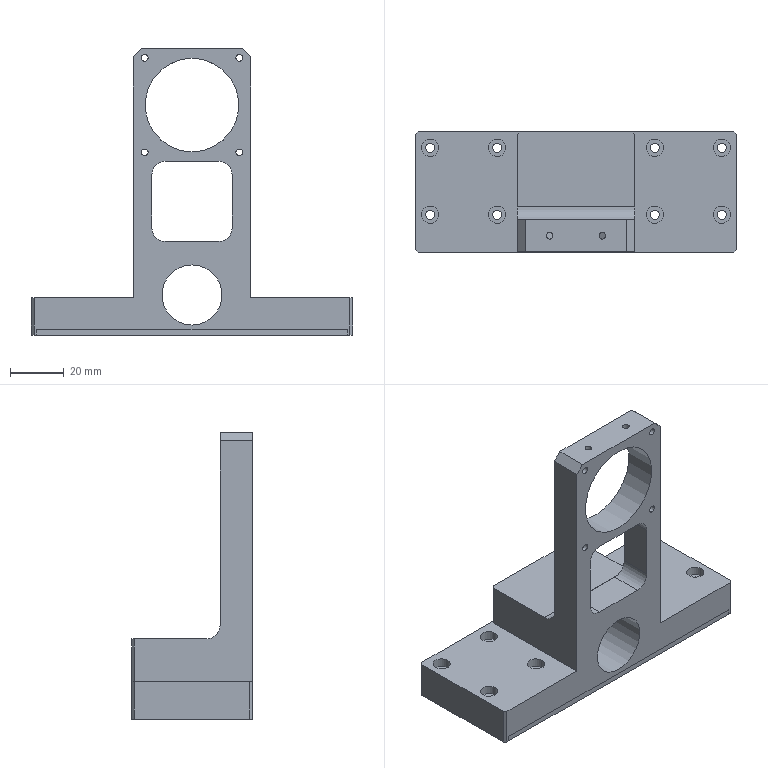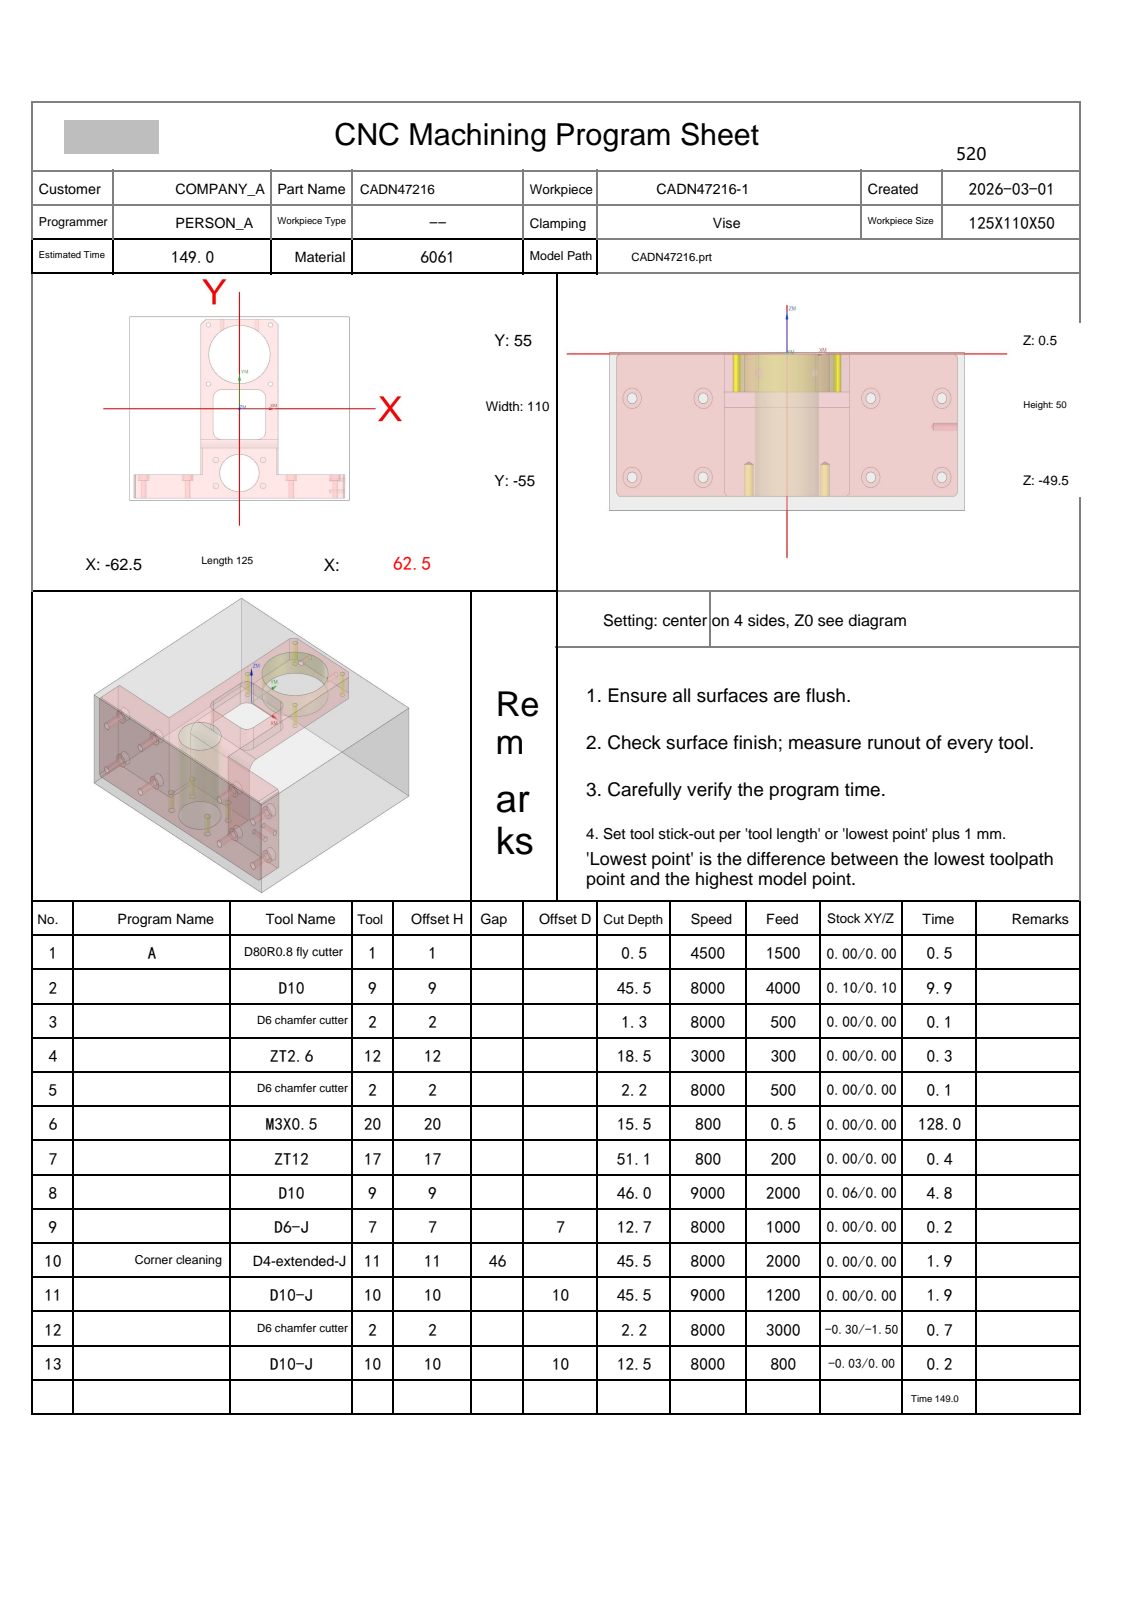NC program | NX | posted by the shop | part box 120 x 45 x 107 mm
Lines 6509 to 7503 of 16292:
N10 T11 M06
(D4-extended-J  D=4. R=0. H=11 ce=0.00 di=0.00)
G00 G90 G54 X-27.403 Y-37.1 M03 S8000
G43 H11 Z50.
M08
Z.15
G01 X-27.402 Y-37.105 Z.089 F2000.
X-27.398 Y-37.119 Z.034
X-27.392 Y-37.142 Z-.014
X-27.383 Y-37.17 Z-.058
X-27.37 Y-37.204 Z-.096
X-27.354 Y-37.241 Z-.129
X-27.334 Y-37.28 Z-.157
X-27.31 Y-37.32 Z-.181
X-27.282 Y-37.359 Z-.201
X-27.249 Y-37.396 Z-.217
X-27.211 Y-37.43 Z-.23
X-27.167 Y-37.458 Z-.239
X-27.119 Y-37.481 Z-.245
X-27.064 Y-37.495 Z-.249
X-27.003 Y-37.5 Z-.25
X-24.
Y-34.497
X-24.014 Y-34.454 Z-.251
X-24.053 Y-34.433 Z-.253
X-24.116 Y-34.432 Z-.256
X-24.199 Y-34.45 Z-.261
X-24.299 Y-34.485 Z-.267
X-24.414 Y-34.535 Z-.274
X-24.541 Y-34.599 Z-.281
X-24.677 Y-34.675 Z-.29
X-24.896 Y-34.812 Z-.303
X-25.113 Y-34.96 Z-.318
X-25.509 Y-35.271 Z-.346
X-25.883 Y-35.617 Z-.375
X-26.229 Y-35.991 Z-.404
X-26.54 Y-36.387 Z-.432
X-26.688 Y-36.604 Z-.447
X-26.825 Y-36.823 Z-.46
X-26.901 Y-36.959 Z-.469
X-26.965 Y-37.086 Z-.476
X-27.015 Y-37.201 Z-.483
X-27.05 Y-37.301 Z-.489
X-27.068 Y-37.384 Z-.494
X-27.067 Y-37.447 Z-.497
X-27.046 Y-37.486 Z-.499
X-27.003 Y-37.5 Z-.5
X-24.
Y-34.497
X-24.014 Y-34.454 Z-.501
X-24.053 Y-34.433 Z-.503
X-24.116 Y-34.432 Z-.506
X-24.199 Y-34.45 Z-.511
X-24.299 Y-34.485 Z-.517
X-24.414 Y-34.535 Z-.524
X-24.541 Y-34.599 Z-.531
X-24.677 Y-34.675 Z-.54
X-24.896 Y-34.812 Z-.553
X-25.113 Y-34.96 Z-.568
X-25.509 Y-35.271 Z-.596
X-25.883 Y-35.617 Z-.625
X-26.229 Y-35.991 Z-.654
X-26.54 Y-36.387 Z-.682
X-26.688 Y-36.604 Z-.697
X-26.825 Y-36.823 Z-.71
X-26.901 Y-36.959 Z-.719
X-26.965 Y-37.086 Z-.726
X-27.015 Y-37.201 Z-.733
X-27.05 Y-37.301 Z-.739
X-27.068 Y-37.384 Z-.744
X-27.067 Y-37.447 Z-.747
X-27.046 Y-37.486 Z-.749
X-27.003 Y-37.5 Z-.75
X-24.
Y-34.497
X-24.014 Y-34.454 Z-.751
X-24.053 Y-34.433 Z-.753
X-24.116 Y-34.432 Z-.756
X-24.199 Y-34.45 Z-.761
X-24.299 Y-34.485 Z-.767
X-24.414 Y-34.535 Z-.774
X-24.541 Y-34.599 Z-.781
X-24.677 Y-34.675 Z-.79
X-24.896 Y-34.812 Z-.803
X-25.113 Y-34.96 Z-.818
X-25.509 Y-35.271 Z-.846
X-25.883 Y-35.617 Z-.875
X-26.229 Y-35.991 Z-.904
X-26.54 Y-36.387 Z-.932
X-26.688 Y-36.604 Z-.947
X-26.825 Y-36.823 Z-.96
X-26.901 Y-36.959 Z-.969
X-26.965 Y-37.086 Z-.976
X-27.015 Y-37.201 Z-.983
X-27.05 Y-37.301 Z-.989
X-27.068 Y-37.384 Z-.994
X-27.067 Y-37.447 Z-.997
X-27.046 Y-37.486 Z-.999
X-27.003 Y-37.5 Z-1.
X-24.
Y-34.497
X-24.014 Y-34.454 Z-1.001
X-24.053 Y-34.433 Z-1.003
X-24.116 Y-34.432 Z-1.006
X-24.199 Y-34.45 Z-1.011
X-24.299 Y-34.485 Z-1.017
X-24.414 Y-34.535 Z-1.024
X-24.541 Y-34.599 Z-1.031
X-24.677 Y-34.675 Z-1.04
X-24.896 Y-34.811 Z-1.053
X-25.113 Y-34.96 Z-1.068
X-25.509 Y-35.271 Z-1.096
X-25.883 Y-35.617 Z-1.125
X-26.229 Y-35.991 Z-1.154
X-26.54 Y-36.386 Z-1.182
X-26.688 Y-36.604 Z-1.197
X-26.825 Y-36.823 Z-1.21
X-26.901 Y-36.959 Z-1.219
X-26.965 Y-37.086 Z-1.226
X-27.015 Y-37.201 Z-1.233
X-27.05 Y-37.301 Z-1.239
X-27.068 Y-37.384 Z-1.244
X-27.067 Y-37.447 Z-1.247
X-27.046 Y-37.486 Z-1.249
X-27.003 Y-37.5 Z-1.25
X-24.
Y-34.497
X-24.014 Y-34.454 Z-1.251
X-24.053 Y-34.433 Z-1.253
X-24.116 Y-34.432 Z-1.256
X-24.199 Y-34.45 Z-1.261
X-24.299 Y-34.485 Z-1.267
X-24.414 Y-34.535 Z-1.274
X-24.541 Y-34.599 Z-1.281
X-24.677 Y-34.675 Z-1.29
X-24.896 Y-34.811 Z-1.303
X-25.113 Y-34.96 Z-1.318
X-25.509 Y-35.271 Z-1.346
X-25.883 Y-35.617 Z-1.375
X-26.229 Y-35.991 Z-1.404
X-26.54 Y-36.386 Z-1.432
X-26.688 Y-36.604 Z-1.447
X-26.825 Y-36.823 Z-1.46
X-26.901 Y-36.959 Z-1.469
X-26.965 Y-37.086 Z-1.476
X-27.015 Y-37.201 Z-1.483
X-27.05 Y-37.301 Z-1.489
X-27.068 Y-37.384 Z-1.494
X-27.067 Y-37.447 Z-1.497
X-27.046 Y-37.486 Z-1.499
X-27.003 Y-37.5 Z-1.5
X-24.
Y-34.497
X-24.014 Y-34.454 Z-1.501
X-24.053 Y-34.433 Z-1.503
X-24.116 Y-34.432 Z-1.506
X-24.199 Y-34.45 Z-1.511
X-24.299 Y-34.485 Z-1.517
X-24.414 Y-34.535 Z-1.524
X-24.541 Y-34.599 Z-1.531
X-24.677 Y-34.675 Z-1.54
X-24.896 Y-34.811 Z-1.553
X-25.113 Y-34.96 Z-1.568
X-25.509 Y-35.271 Z-1.596
X-25.883 Y-35.617 Z-1.625
X-26.229 Y-35.991 Z-1.654
X-26.54 Y-36.386 Z-1.682
X-26.688 Y-36.604 Z-1.697
X-26.825 Y-36.823 Z-1.71
X-26.901 Y-36.959 Z-1.719
X-26.965 Y-37.086 Z-1.726
X-27.015 Y-37.201 Z-1.733
X-27.05 Y-37.301 Z-1.739
X-27.068 Y-37.384 Z-1.744
X-27.067 Y-37.447 Z-1.747
X-27.046 Y-37.486 Z-1.749
X-27.003 Y-37.5 Z-1.75
X-24.
Y-34.497
X-24.014 Y-34.454 Z-1.751
X-24.053 Y-34.433 Z-1.753
X-24.116 Y-34.432 Z-1.756
X-24.199 Y-34.45 Z-1.761
X-24.299 Y-34.485 Z-1.767
X-24.414 Y-34.535 Z-1.774
X-24.541 Y-34.599 Z-1.781
X-24.677 Y-34.675 Z-1.79
X-24.896 Y-34.811 Z-1.803
X-25.113 Y-34.96 Z-1.818
X-25.509 Y-35.271 Z-1.846
X-25.883 Y-35.617 Z-1.875
X-26.229 Y-35.991 Z-1.904
X-26.54 Y-36.386 Z-1.932
X-26.688 Y-36.604 Z-1.947
X-26.825 Y-36.823 Z-1.96
X-26.901 Y-36.959 Z-1.969
X-26.965 Y-37.086 Z-1.976
X-27.015 Y-37.201 Z-1.983
X-27.05 Y-37.301 Z-1.989
X-27.068 Y-37.384 Z-1.994
X-27.067 Y-37.447 Z-1.997
X-27.046 Y-37.486 Z-1.999
X-27.003 Y-37.5 Z-2.
X-24.
Y-34.497
X-24.014 Y-34.454 Z-2.001
X-24.053 Y-34.433 Z-2.003
X-24.116 Y-34.432 Z-2.006
X-24.199 Y-34.45 Z-2.011
X-24.299 Y-34.485 Z-2.017
X-24.414 Y-34.535 Z-2.024
X-24.541 Y-34.599 Z-2.031
X-24.677 Y-34.675 Z-2.04
X-24.896 Y-34.811 Z-2.053
X-25.113 Y-34.96 Z-2.068
X-25.509 Y-35.271 Z-2.096
X-25.883 Y-35.617 Z-2.125
X-26.229 Y-35.991 Z-2.154
X-26.54 Y-36.386 Z-2.182
X-26.688 Y-36.604 Z-2.197
X-26.825 Y-36.823 Z-2.21
X-26.901 Y-36.959 Z-2.219
X-26.965 Y-37.086 Z-2.226
X-27.015 Y-37.201 Z-2.233
X-27.05 Y-37.301 Z-2.239
X-27.068 Y-37.384 Z-2.244
X-27.067 Y-37.447 Z-2.247
X-27.046 Y-37.486 Z-2.249
X-27.003 Y-37.5 Z-2.25
X-24.
Y-34.497
X-24.014 Y-34.454 Z-2.251
X-24.053 Y-34.433 Z-2.253
X-24.116 Y-34.432 Z-2.256
X-24.199 Y-34.45 Z-2.261
X-24.299 Y-34.485 Z-2.267
X-24.414 Y-34.535 Z-2.274
X-24.541 Y-34.599 Z-2.281
X-24.677 Y-34.675 Z-2.29
X-24.896 Y-34.811 Z-2.303
X-25.113 Y-34.96 Z-2.318
X-25.509 Y-35.271 Z-2.346
X-25.883 Y-35.617 Z-2.375
X-26.229 Y-35.991 Z-2.404
X-26.54 Y-36.386 Z-2.432
X-26.688 Y-36.604 Z-2.447
X-26.825 Y-36.823 Z-2.46
X-26.901 Y-36.959 Z-2.469
X-26.965 Y-37.086 Z-2.476
X-27.015 Y-37.201 Z-2.483
X-27.05 Y-37.301 Z-2.489
X-27.068 Y-37.384 Z-2.494
X-27.067 Y-37.447 Z-2.497
X-27.046 Y-37.486 Z-2.499
X-27.003 Y-37.5 Z-2.5
X-24.
Y-34.497
X-24.014 Y-34.454 Z-2.501
X-24.053 Y-34.433 Z-2.503
X-24.116 Y-34.432 Z-2.506
X-24.199 Y-34.45 Z-2.511
X-24.299 Y-34.485 Z-2.517
X-24.414 Y-34.535 Z-2.524
X-24.541 Y-34.599 Z-2.531
X-24.677 Y-34.675 Z-2.54
X-24.896 Y-34.811 Z-2.553
X-25.113 Y-34.96 Z-2.568
X-25.509 Y-35.271 Z-2.596
X-25.883 Y-35.617 Z-2.625
X-26.229 Y-35.991 Z-2.654
X-26.54 Y-36.386 Z-2.682
X-26.688 Y-36.604 Z-2.697
X-26.825 Y-36.823 Z-2.71
X-26.901 Y-36.959 Z-2.719
X-26.965 Y-37.086 Z-2.726
X-27.015 Y-37.201 Z-2.733
X-27.05 Y-37.301 Z-2.739
X-27.068 Y-37.384 Z-2.744
X-27.067 Y-37.447 Z-2.747
X-27.046 Y-37.486 Z-2.749
X-27.003 Y-37.5 Z-2.75
X-24.
Y-34.497
X-24.014 Y-34.454 Z-2.751
X-24.053 Y-34.433 Z-2.753
X-24.116 Y-34.432 Z-2.756
X-24.199 Y-34.45 Z-2.761
X-24.299 Y-34.485 Z-2.767
X-24.414 Y-34.535 Z-2.774
X-24.541 Y-34.599 Z-2.781
X-24.677 Y-34.675 Z-2.79
X-24.896 Y-34.811 Z-2.803
X-25.113 Y-34.96 Z-2.818
X-25.509 Y-35.271 Z-2.846
X-25.883 Y-35.617 Z-2.875
X-26.229 Y-35.991 Z-2.904
X-26.54 Y-36.386 Z-2.932
X-26.688 Y-36.604 Z-2.947
X-26.825 Y-36.823 Z-2.96
X-26.901 Y-36.959 Z-2.969
X-26.965 Y-37.086 Z-2.976
X-27.015 Y-37.201 Z-2.983
X-27.05 Y-37.301 Z-2.989
X-27.068 Y-37.384 Z-2.994
X-27.067 Y-37.447 Z-2.997
X-27.046 Y-37.486 Z-2.999
X-27.003 Y-37.5 Z-3.
X-24.
Y-34.497
X-24.014 Y-34.454 Z-3.001
X-24.053 Y-34.433 Z-3.003
X-24.116 Y-34.432 Z-3.006
X-24.199 Y-34.45 Z-3.011
X-24.299 Y-34.485 Z-3.017
X-24.414 Y-34.535 Z-3.024
X-24.541 Y-34.599 Z-3.031
X-24.677 Y-34.675 Z-3.04
X-24.896 Y-34.811 Z-3.053
X-25.113 Y-34.96 Z-3.068
X-25.509 Y-35.271 Z-3.096
X-25.883 Y-35.617 Z-3.125
X-26.229 Y-35.991 Z-3.154
X-26.54 Y-36.386 Z-3.182
X-26.688 Y-36.604 Z-3.197
X-26.825 Y-36.823 Z-3.21
X-26.901 Y-36.959 Z-3.219
X-26.965 Y-37.086 Z-3.226
X-27.015 Y-37.201 Z-3.233
X-27.05 Y-37.301 Z-3.239
X-27.068 Y-37.384 Z-3.244
X-27.067 Y-37.447 Z-3.247
X-27.046 Y-37.486 Z-3.249
X-27.003 Y-37.5 Z-3.25
X-24.
Y-34.497
X-24.014 Y-34.454 Z-3.251
X-24.053 Y-34.433 Z-3.253
X-24.116 Y-34.432 Z-3.256
X-24.199 Y-34.45 Z-3.261
X-24.299 Y-34.485 Z-3.267
X-24.414 Y-34.535 Z-3.274
X-24.541 Y-34.599 Z-3.281
X-24.677 Y-34.675 Z-3.29
X-24.896 Y-34.811 Z-3.303
X-25.113 Y-34.96 Z-3.318
X-25.509 Y-35.271 Z-3.346
X-25.883 Y-35.617 Z-3.375
X-26.229 Y-35.991 Z-3.404
X-26.54 Y-36.386 Z-3.432
X-26.688 Y-36.604 Z-3.447
X-26.825 Y-36.823 Z-3.46
X-26.901 Y-36.959 Z-3.469
X-26.965 Y-37.086 Z-3.476
X-27.015 Y-37.201 Z-3.483
X-27.05 Y-37.301 Z-3.489
X-27.068 Y-37.384 Z-3.494
X-27.067 Y-37.447 Z-3.497
X-27.046 Y-37.486 Z-3.499
X-27.003 Y-37.5 Z-3.5
X-24.
Y-34.497
X-24.014 Y-34.454 Z-3.501
X-24.053 Y-34.433 Z-3.503
X-24.116 Y-34.432 Z-3.506
X-24.199 Y-34.45 Z-3.511
X-24.299 Y-34.485 Z-3.517
X-24.414 Y-34.535 Z-3.524
X-24.541 Y-34.599 Z-3.531
X-24.677 Y-34.675 Z-3.54
X-24.896 Y-34.811 Z-3.553
X-25.113 Y-34.96 Z-3.568
X-25.509 Y-35.271 Z-3.596
X-25.883 Y-35.617 Z-3.625
X-26.229 Y-35.991 Z-3.654
X-26.54 Y-36.386 Z-3.682
X-26.688 Y-36.604 Z-3.697
X-26.825 Y-36.823 Z-3.71
X-26.901 Y-36.959 Z-3.719
X-26.965 Y-37.086 Z-3.726
X-27.015 Y-37.201 Z-3.733
X-27.05 Y-37.301 Z-3.739
X-27.068 Y-37.384 Z-3.744
X-27.067 Y-37.447 Z-3.747
X-27.046 Y-37.486 Z-3.749
X-27.003 Y-37.5 Z-3.75
X-24.
Y-34.497
X-24.014 Y-34.454 Z-3.751
X-24.053 Y-34.433 Z-3.753
X-24.116 Y-34.432 Z-3.756
X-24.199 Y-34.45 Z-3.761
X-24.299 Y-34.485 Z-3.767
X-24.414 Y-34.535 Z-3.774
X-24.541 Y-34.599 Z-3.781
X-24.677 Y-34.675 Z-3.79
X-24.896 Y-34.811 Z-3.803
X-25.113 Y-34.96 Z-3.818
X-25.509 Y-35.271 Z-3.846
X-25.883 Y-35.617 Z-3.875
X-26.229 Y-35.991 Z-3.904
X-26.54 Y-36.386 Z-3.932
X-26.688 Y-36.604 Z-3.947
X-26.825 Y-36.823 Z-3.96
X-26.901 Y-36.959 Z-3.969
X-26.965 Y-37.086 Z-3.976
X-27.015 Y-37.201 Z-3.983
X-27.05 Y-37.301 Z-3.989
X-27.068 Y-37.384 Z-3.994
X-27.067 Y-37.447 Z-3.997
X-27.046 Y-37.486 Z-3.999
X-27.003 Y-37.5 Z-4.
X-24.
Y-34.497
X-24.014 Y-34.454 Z-4.001
X-24.053 Y-34.433 Z-4.003
X-24.116 Y-34.432 Z-4.006
X-24.199 Y-34.45 Z-4.011
X-24.299 Y-34.485 Z-4.017
X-24.414 Y-34.535 Z-4.024
X-24.541 Y-34.599 Z-4.031
X-24.677 Y-34.675 Z-4.04
X-24.896 Y-34.811 Z-4.053
X-25.113 Y-34.96 Z-4.068
X-25.509 Y-35.271 Z-4.096
X-25.883 Y-35.617 Z-4.125
X-26.229 Y-35.991 Z-4.154
X-26.54 Y-36.386 Z-4.182
X-26.688 Y-36.604 Z-4.197
X-26.825 Y-36.823 Z-4.21
X-26.901 Y-36.959 Z-4.219
X-26.965 Y-37.086 Z-4.226
X-27.015 Y-37.201 Z-4.233
X-27.05 Y-37.301 Z-4.239
X-27.068 Y-37.384 Z-4.244
X-27.067 Y-37.447 Z-4.247
X-27.046 Y-37.486 Z-4.249
X-27.003 Y-37.5 Z-4.25
X-24.
Y-34.497
X-24.014 Y-34.454 Z-4.251
X-24.053 Y-34.433 Z-4.253
X-24.116 Y-34.432 Z-4.256
X-24.199 Y-34.45 Z-4.261
X-24.299 Y-34.485 Z-4.267
X-24.414 Y-34.535 Z-4.274
X-24.541 Y-34.599 Z-4.281
X-24.677 Y-34.675 Z-4.29
X-24.896 Y-34.811 Z-4.303
X-25.113 Y-34.96 Z-4.318
X-25.509 Y-35.271 Z-4.346
X-25.883 Y-35.617 Z-4.375
X-26.229 Y-35.991 Z-4.404
X-26.54 Y-36.386 Z-4.432
X-26.688 Y-36.604 Z-4.447
X-26.825 Y-36.823 Z-4.46
X-26.901 Y-36.959 Z-4.469
X-26.965 Y-37.086 Z-4.476
X-27.015 Y-37.201 Z-4.483
X-27.05 Y-37.301 Z-4.489
X-27.068 Y-37.384 Z-4.494
X-27.067 Y-37.447 Z-4.497
X-27.046 Y-37.486 Z-4.499
X-27.003 Y-37.5 Z-4.5
X-24.
Y-34.497
X-24.014 Y-34.454 Z-4.501
X-24.053 Y-34.433 Z-4.503
X-24.116 Y-34.432 Z-4.506
X-24.199 Y-34.45 Z-4.511
X-24.299 Y-34.485 Z-4.517
X-24.414 Y-34.535 Z-4.524
X-24.541 Y-34.599 Z-4.531
X-24.677 Y-34.675 Z-4.54
X-24.896 Y-34.811 Z-4.553
X-25.113 Y-34.96 Z-4.568
X-25.509 Y-35.271 Z-4.596
X-25.883 Y-35.617 Z-4.625
X-26.229 Y-35.991 Z-4.654
X-26.54 Y-36.386 Z-4.682
X-26.688 Y-36.604 Z-4.697
X-26.825 Y-36.823 Z-4.71
X-26.901 Y-36.959 Z-4.719
X-26.965 Y-37.086 Z-4.726
X-27.015 Y-37.201 Z-4.733
X-27.05 Y-37.301 Z-4.739
X-27.068 Y-37.384 Z-4.744
X-27.067 Y-37.447 Z-4.747
X-27.046 Y-37.486 Z-4.749
X-27.003 Y-37.5 Z-4.75
X-24.
Y-34.497
X-24.014 Y-34.454 Z-4.751
X-24.053 Y-34.433 Z-4.753
X-24.116 Y-34.432 Z-4.756
X-24.199 Y-34.45 Z-4.761
X-24.299 Y-34.485 Z-4.767
X-24.414 Y-34.535 Z-4.774
X-24.541 Y-34.599 Z-4.781
X-24.677 Y-34.675 Z-4.79
X-24.896 Y-34.811 Z-4.803
X-25.113 Y-34.96 Z-4.818
X-25.509 Y-35.271 Z-4.846
X-25.883 Y-35.617 Z-4.875
X-26.229 Y-35.991 Z-4.904
X-26.54 Y-36.386 Z-4.932
X-26.688 Y-36.604 Z-4.947
X-26.825 Y-36.823 Z-4.96
X-26.901 Y-36.959 Z-4.969
X-26.965 Y-37.086 Z-4.976
X-27.015 Y-37.201 Z-4.983
X-27.05 Y-37.301 Z-4.989
X-27.068 Y-37.384 Z-4.994
X-27.067 Y-37.447 Z-4.997
X-27.046 Y-37.486 Z-4.999
X-27.003 Y-37.5 Z-5.
X-24.
Y-34.497
X-24.014 Y-34.454 Z-5.001
X-24.053 Y-34.433 Z-5.003
X-24.116 Y-34.432 Z-5.006
X-24.199 Y-34.45 Z-5.011
X-24.299 Y-34.485 Z-5.017
X-24.414 Y-34.535 Z-5.024
X-24.541 Y-34.599 Z-5.031
X-24.677 Y-34.675 Z-5.04
X-24.896 Y-34.811 Z-5.053
X-25.113 Y-34.96 Z-5.068
X-25.509 Y-35.271 Z-5.096
X-25.883 Y-35.617 Z-5.125
X-26.229 Y-35.991 Z-5.154
X-26.54 Y-36.386 Z-5.182
X-26.688 Y-36.604 Z-5.197
X-26.825 Y-36.823 Z-5.21
X-26.901 Y-36.959 Z-5.219
X-26.965 Y-37.086 Z-5.226
X-27.015 Y-37.201 Z-5.233
X-27.05 Y-37.301 Z-5.239
X-27.068 Y-37.384 Z-5.244
X-27.067 Y-37.447 Z-5.247
X-27.046 Y-37.486 Z-5.249
X-27.003 Y-37.5 Z-5.25
X-24.
Y-34.497
X-24.014 Y-34.454 Z-5.251
X-24.053 Y-34.433 Z-5.253
X-24.116 Y-34.432 Z-5.256
X-24.199 Y-34.45 Z-5.261
X-24.299 Y-34.485 Z-5.267
X-24.414 Y-34.535 Z-5.274
X-24.541 Y-34.599 Z-5.281
X-24.677 Y-34.675 Z-5.29
X-24.896 Y-34.811 Z-5.303
X-25.113 Y-34.96 Z-5.318
X-25.509 Y-35.271 Z-5.346
X-25.883 Y-35.617 Z-5.375
X-26.229 Y-35.991 Z-5.404
X-26.54 Y-36.386 Z-5.432
X-26.688 Y-36.604 Z-5.447
X-26.825 Y-36.823 Z-5.46
X-26.901 Y-36.959 Z-5.469
X-26.965 Y-37.086 Z-5.476
X-27.015 Y-37.201 Z-5.483
X-27.05 Y-37.301 Z-5.489
X-27.068 Y-37.384 Z-5.494
X-27.067 Y-37.447 Z-5.497
X-27.046 Y-37.486 Z-5.499
X-27.003 Y-37.5 Z-5.5
X-24.
Y-34.497
X-24.014 Y-34.454 Z-5.501
X-24.053 Y-34.433 Z-5.503
X-24.116 Y-34.432 Z-5.506
X-24.199 Y-34.45 Z-5.511
X-24.299 Y-34.485 Z-5.517
X-24.414 Y-34.535 Z-5.524
X-24.541 Y-34.599 Z-5.531
X-24.677 Y-34.675 Z-5.54
X-24.896 Y-34.811 Z-5.553
X-25.113 Y-34.96 Z-5.568
X-25.509 Y-35.271 Z-5.596
X-25.883 Y-35.617 Z-5.625
X-26.229 Y-35.991 Z-5.654
X-26.54 Y-36.386 Z-5.682
X-26.688 Y-36.604 Z-5.697
X-26.825 Y-36.823 Z-5.71
X-26.901 Y-36.959 Z-5.719
X-26.965 Y-37.086 Z-5.726
X-27.015 Y-37.201 Z-5.733
X-27.05 Y-37.301 Z-5.739
X-27.068 Y-37.384 Z-5.744
X-27.067 Y-37.447 Z-5.747
X-27.046 Y-37.486 Z-5.749
X-27.003 Y-37.5 Z-5.75
X-24.
Y-34.497
X-24.014 Y-34.454 Z-5.751
X-24.053 Y-34.433 Z-5.753
X-24.116 Y-34.432 Z-5.756
X-24.199 Y-34.45 Z-5.761
X-24.299 Y-34.485 Z-5.767
X-24.414 Y-34.535 Z-5.774
X-24.541 Y-34.599 Z-5.781
X-24.677 Y-34.675 Z-5.79
X-24.896 Y-34.811 Z-5.803
X-25.113 Y-34.96 Z-5.818
X-25.509 Y-35.271 Z-5.846
X-25.883 Y-35.617 Z-5.875
X-26.229 Y-35.991 Z-5.904
X-26.54 Y-36.386 Z-5.932
X-26.688 Y-36.604 Z-5.947
X-26.825 Y-36.823 Z-5.96
X-26.901 Y-36.959 Z-5.969
X-26.965 Y-37.086 Z-5.976
X-27.015 Y-37.201 Z-5.983
X-27.05 Y-37.301 Z-5.989
X-27.068 Y-37.384 Z-5.994
X-27.067 Y-37.447 Z-5.997
X-27.046 Y-37.486 Z-5.999
X-27.003 Y-37.5 Z-6.
X-24.
Y-34.497
X-24.014 Y-34.454 Z-6.001
X-24.053 Y-34.433 Z-6.003
X-24.116 Y-34.432 Z-6.006
X-24.199 Y-34.45 Z-6.011
X-24.299 Y-34.485 Z-6.017
X-24.414 Y-34.535 Z-6.024
X-24.541 Y-34.599 Z-6.031
X-24.677 Y-34.675 Z-6.04
X-24.896 Y-34.811 Z-6.053
X-25.113 Y-34.96 Z-6.068
X-25.509 Y-35.271 Z-6.096
X-25.883 Y-35.617 Z-6.125
X-26.229 Y-35.991 Z-6.154
X-26.54 Y-36.386 Z-6.182
X-26.688 Y-36.604 Z-6.197
X-26.825 Y-36.823 Z-6.21
X-26.901 Y-36.959 Z-6.219
X-26.965 Y-37.086 Z-6.226
X-27.015 Y-37.201 Z-6.233
X-27.05 Y-37.301 Z-6.239
X-27.068 Y-37.384 Z-6.244
X-27.067 Y-37.447 Z-6.247
X-27.046 Y-37.486 Z-6.249
X-27.003 Y-37.5 Z-6.25
X-24.
Y-34.497
X-24.014 Y-34.454 Z-6.251
X-24.053 Y-34.433 Z-6.253
X-24.116 Y-34.432 Z-6.256
X-24.199 Y-34.45 Z-6.261
X-24.299 Y-34.485 Z-6.267
X-24.414 Y-34.535 Z-6.274
X-24.541 Y-34.599 Z-6.281
X-24.677 Y-34.675 Z-6.29
X-24.896 Y-34.811 Z-6.303
X-25.113 Y-34.96 Z-6.318
X-25.509 Y-35.271 Z-6.346
X-25.883 Y-35.617 Z-6.375
X-26.229 Y-35.991 Z-6.404
X-26.54 Y-36.386 Z-6.432
X-26.688 Y-36.604 Z-6.447
X-26.825 Y-36.823 Z-6.46
X-26.901 Y-36.959 Z-6.469
X-26.965 Y-37.086 Z-6.476
X-27.015 Y-37.201 Z-6.483
X-27.05 Y-37.301 Z-6.489
X-27.068 Y-37.384 Z-6.494
X-27.067 Y-37.447 Z-6.497
X-27.046 Y-37.486 Z-6.499
X-27.003 Y-37.5 Z-6.5
X-24.
Y-34.497
X-24.014 Y-34.454 Z-6.501
X-24.053 Y-34.433 Z-6.503
X-24.116 Y-34.432 Z-6.506
X-24.199 Y-34.45 Z-6.511
X-24.299 Y-34.485 Z-6.517
X-24.414 Y-34.535 Z-6.524
X-24.541 Y-34.599 Z-6.531
X-24.677 Y-34.675 Z-6.54
X-24.896 Y-34.811 Z-6.553
X-25.113 Y-34.96 Z-6.568
X-25.509 Y-35.271 Z-6.596
X-25.883 Y-35.617 Z-6.625
X-26.229 Y-35.991 Z-6.654
X-26.54 Y-36.386 Z-6.682
X-26.688 Y-36.604 Z-6.697
X-26.825 Y-36.823 Z-6.71
X-26.901 Y-36.959 Z-6.719
X-26.965 Y-37.086 Z-6.726
X-27.015 Y-37.201 Z-6.733
X-27.05 Y-37.301 Z-6.739
X-27.068 Y-37.384 Z-6.744
X-27.067 Y-37.447 Z-6.747
X-27.046 Y-37.486 Z-6.749
X-27.003 Y-37.5 Z-6.75
X-24.
Y-34.497
X-24.014 Y-34.454 Z-6.751
X-24.053 Y-34.433 Z-6.753
X-24.116 Y-34.432 Z-6.756
X-24.199 Y-34.45 Z-6.761
X-24.299 Y-34.485 Z-6.767
X-24.414 Y-34.535 Z-6.774
X-24.541 Y-34.599 Z-6.781
X-24.677 Y-34.675 Z-6.79
X-24.896 Y-34.811 Z-6.803
X-25.113 Y-34.96 Z-6.818
X-25.509 Y-35.271 Z-6.846
X-25.883 Y-35.617 Z-6.875
X-26.229 Y-35.991 Z-6.904
X-26.54 Y-36.386 Z-6.932
X-26.688 Y-36.604 Z-6.947
X-26.825 Y-36.823 Z-6.96
X-26.901 Y-36.959 Z-6.969
X-26.965 Y-37.086 Z-6.976
X-27.015 Y-37.201 Z-6.983
X-27.05 Y-37.301 Z-6.989
X-27.068 Y-37.384 Z-6.994
X-27.067 Y-37.447 Z-6.997
X-27.046 Y-37.486 Z-6.999
X-27.003 Y-37.5 Z-7.
X-24.
Y-34.497
X-24.014 Y-34.454 Z-7.001
X-24.053 Y-34.433 Z-7.003
X-24.116 Y-34.432 Z-7.006
X-24.199 Y-34.45 Z-7.011
X-24.299 Y-34.485 Z-7.017
X-24.414 Y-34.535 Z-7.024
X-24.541 Y-34.599 Z-7.031
X-24.677 Y-34.675 Z-7.04
X-24.896 Y-34.811 Z-7.053
X-25.113 Y-34.96 Z-7.068
X-25.509 Y-35.271 Z-7.096
X-25.883 Y-35.617 Z-7.125
X-26.229 Y-35.991 Z-7.154
X-26.54 Y-36.386 Z-7.182
X-26.688 Y-36.604 Z-7.197
X-26.825 Y-36.823 Z-7.21
X-26.901 Y-36.959 Z-7.219
X-26.965 Y-37.086 Z-7.226
X-27.015 Y-37.201 Z-7.233
X-27.05 Y-37.301 Z-7.239
X-27.068 Y-37.384 Z-7.244
X-27.067 Y-37.447 Z-7.247
X-27.046 Y-37.486 Z-7.249
X-27.003 Y-37.5 Z-7.25
X-24.
Y-34.497
X-24.014 Y-34.454 Z-7.251
X-24.053 Y-34.433 Z-7.253
X-24.116 Y-34.432 Z-7.256
X-24.199 Y-34.45 Z-7.261
X-24.299 Y-34.485 Z-7.267
X-24.414 Y-34.535 Z-7.274
X-24.541 Y-34.599 Z-7.281
X-24.677 Y-34.675 Z-7.29
X-24.896 Y-34.811 Z-7.303
X-25.113 Y-34.96 Z-7.318
X-25.509 Y-35.271 Z-7.346
X-25.883 Y-35.617 Z-7.375
X-26.229 Y-35.991 Z-7.404
X-26.54 Y-36.386 Z-7.432
X-26.688 Y-36.604 Z-7.447
X-26.825 Y-36.823 Z-7.46
X-26.901 Y-36.959 Z-7.469
X-26.965 Y-37.086 Z-7.476
X-27.015 Y-37.201 Z-7.483
X-27.05 Y-37.301 Z-7.489
X-27.068 Y-37.384 Z-7.494
X-27.067 Y-37.447 Z-7.497
X-27.046 Y-37.486 Z-7.499
X-27.003 Y-37.5 Z-7.5
X-24.
Y-34.497
X-24.014 Y-34.454 Z-7.501
X-24.053 Y-34.433 Z-7.503
X-24.116 Y-34.432 Z-7.506
X-24.199 Y-34.45 Z-7.511
X-24.299 Y-34.485 Z-7.517
X-24.414 Y-34.535 Z-7.524
X-24.541 Y-34.599 Z-7.531
X-24.677 Y-34.675 Z-7.54
X-24.896 Y-34.811 Z-7.553
X-25.113 Y-34.96 Z-7.568
X-25.509 Y-35.271 Z-7.596
X-25.883 Y-35.617 Z-7.625
X-26.229 Y-35.991 Z-7.654
X-26.54 Y-36.386 Z-7.682
X-26.688 Y-36.604 Z-7.697
X-26.825 Y-36.823 Z-7.71
X-26.901 Y-36.959 Z-7.719
X-26.965 Y-37.086 Z-7.726
X-27.015 Y-37.201 Z-7.733
X-27.05 Y-37.301 Z-7.739
X-27.068 Y-37.384 Z-7.744
X-27.067 Y-37.447 Z-7.747
X-27.046 Y-37.486 Z-7.749
X-27.003 Y-37.5 Z-7.75
X-24.
Y-34.497
X-24.014 Y-34.454 Z-7.751
X-24.053 Y-34.433 Z-7.753
X-24.116 Y-34.432 Z-7.756
X-24.199 Y-34.45 Z-7.761
X-24.299 Y-34.485 Z-7.767
X-24.414 Y-34.535 Z-7.774
X-24.541 Y-34.599 Z-7.781
X-24.677 Y-34.675 Z-7.79
X-24.896 Y-34.811 Z-7.803
X-25.113 Y-34.96 Z-7.818
X-25.509 Y-35.271 Z-7.846
X-25.883 Y-35.617 Z-7.875
X-26.229 Y-35.991 Z-7.904
X-26.54 Y-36.386 Z-7.932
X-26.688 Y-36.604 Z-7.947
X-26.825 Y-36.823 Z-7.96
X-26.901 Y-36.959 Z-7.969
X-26.965 Y-37.086 Z-7.976
X-27.015 Y-37.201 Z-7.983
X-27.05 Y-37.301 Z-7.989
X-27.068 Y-37.384 Z-7.994
X-27.067 Y-37.447 Z-7.997
X-27.046 Y-37.486 Z-7.999
X-27.003 Y-37.5 Z-8.
X-24.
Y-34.497
X-24.014 Y-34.454 Z-8.001
X-24.053 Y-34.433 Z-8.003
X-24.116 Y-34.432 Z-8.006
X-24.199 Y-34.45 Z-8.011
X-24.299 Y-34.485 Z-8.017
X-24.414 Y-34.535 Z-8.024
X-24.541 Y-34.599 Z-8.031
X-24.677 Y-34.675 Z-8.04
X-24.896 Y-34.811 Z-8.053
X-25.113 Y-34.96 Z-8.068
X-25.509 Y-35.271 Z-8.096
X-25.883 Y-35.617 Z-8.125
X-26.229 Y-35.991 Z-8.154
X-26.54 Y-36.386 Z-8.182
X-26.688 Y-36.604 Z-8.197
X-26.825 Y-36.823 Z-8.21
X-26.901 Y-36.959 Z-8.219
X-26.965 Y-37.086 Z-8.226
X-27.015 Y-37.201 Z-8.233
X-27.05 Y-37.301 Z-8.239
X-27.068 Y-37.384 Z-8.244
X-27.067 Y-37.447 Z-8.247
X-27.046 Y-37.486 Z-8.249
X-27.003 Y-37.5 Z-8.25
X-24.
Y-34.497
X-24.014 Y-34.454 Z-8.251
X-24.053 Y-34.433 Z-8.253
X-24.116 Y-34.432 Z-8.256
X-24.199 Y-34.45 Z-8.261
X-24.299 Y-34.485 Z-8.267
X-24.414 Y-34.535 Z-8.274
X-24.541 Y-34.599 Z-8.281
X-24.677 Y-34.675 Z-8.29
X-24.896 Y-34.811 Z-8.303
X-25.113 Y-34.96 Z-8.318
X-25.509 Y-35.271 Z-8.346
X-25.883 Y-35.617 Z-8.375
X-26.229 Y-35.991 Z-8.404
X-26.54 Y-36.386 Z-8.432
X-26.688 Y-36.604 Z-8.447
X-26.825 Y-36.823 Z-8.46
X-26.901 Y-36.959 Z-8.469
X-26.965 Y-37.086 Z-8.476
X-27.015 Y-37.201 Z-8.483
X-27.05 Y-37.301 Z-8.489
X-27.068 Y-37.384 Z-8.494
X-27.067 Y-37.447 Z-8.497
X-27.046 Y-37.486 Z-8.499
X-27.003 Y-37.5 Z-8.5
X-24.
Y-34.497
X-24.014 Y-34.454 Z-8.501
X-24.053 Y-34.433 Z-8.503
X-24.116 Y-34.432 Z-8.506
X-24.199 Y-34.45 Z-8.511
X-24.299 Y-34.485 Z-8.517
X-24.414 Y-34.535 Z-8.524
X-24.541 Y-34.599 Z-8.531
X-24.677 Y-34.675 Z-8.54
X-24.896 Y-34.811 Z-8.553
X-25.113 Y-34.96 Z-8.568
X-25.509 Y-35.271 Z-8.596
X-25.883 Y-35.617 Z-8.625
X-26.229 Y-35.991 Z-8.654
X-26.54 Y-36.386 Z-8.682
X-26.688 Y-36.604 Z-8.697
X-26.825 Y-36.823 Z-8.71
X-26.901 Y-36.959 Z-8.719
X-26.965 Y-37.086 Z-8.726
X-27.015 Y-37.201 Z-8.733
X-27.05 Y-37.301 Z-8.739
X-27.068 Y-37.384 Z-8.744
X-27.067 Y-37.447 Z-8.747
X-27.046 Y-37.486 Z-8.749
X-27.003 Y-37.5 Z-8.75
X-24.
Y-34.497
X-24.014 Y-34.454 Z-8.751
X-24.053 Y-34.433 Z-8.753
X-24.116 Y-34.432 Z-8.756
X-24.199 Y-34.45 Z-8.761
X-24.299 Y-34.485 Z-8.767
X-24.414 Y-34.535 Z-8.774
X-24.541 Y-34.599 Z-8.781
X-24.677 Y-34.675 Z-8.79
X-24.896 Y-34.811 Z-8.803
X-25.113 Y-34.96 Z-8.818
X-25.509 Y-35.271 Z-8.846
X-25.883 Y-35.617 Z-8.875
X-26.229 Y-35.991 Z-8.904
X-26.54 Y-36.386 Z-8.932
X-26.688 Y-36.604 Z-8.947
X-26.825 Y-36.823 Z-8.96
X-26.901 Y-36.959 Z-8.969
X-26.965 Y-37.086 Z-8.976
X-27.015 Y-37.201 Z-8.983
X-27.05 Y-37.301 Z-8.989
X-27.068 Y-37.384 Z-8.994
X-27.067 Y-37.447 Z-8.997
X-27.046 Y-37.486 Z-8.999
X-27.003 Y-37.5 Z-9.
X-24.
Y-34.497
X-24.014 Y-34.454 Z-9.001
X-24.053 Y-34.433 Z-9.003
X-24.116 Y-34.432 Z-9.006
X-24.199 Y-34.45 Z-9.011
X-24.299 Y-34.485 Z-9.017
X-24.414 Y-34.535 Z-9.024
X-24.541 Y-34.599 Z-9.031
X-24.677 Y-34.675 Z-9.04
X-24.896 Y-34.811 Z-9.053
X-25.113 Y-34.96 Z-9.068
X-25.509 Y-35.271 Z-9.096
X-25.883 Y-35.617 Z-9.125
X-26.229 Y-35.991 Z-9.154
X-26.54 Y-36.386 Z-9.182
X-26.688 Y-36.604 Z-9.197
X-26.825 Y-36.823 Z-9.21
X-26.901 Y-36.959 Z-9.219
X-26.965 Y-37.086 Z-9.226
X-27.015 Y-37.201 Z-9.233
X-27.05 Y-37.301 Z-9.239
X-27.068 Y-37.384 Z-9.244
X-27.067 Y-37.447 Z-9.247
X-27.046 Y-37.486 Z-9.249
X-27.003 Y-37.5 Z-9.25
X-24.
Y-34.497
X-24.014 Y-34.454 Z-9.251
X-24.053 Y-34.433 Z-9.253
X-24.116 Y-34.432 Z-9.256
X-24.199 Y-34.45 Z-9.261
X-24.299 Y-34.485 Z-9.267
X-24.414 Y-34.535 Z-9.274
X-24.541 Y-34.599 Z-9.281
X-24.677 Y-34.675 Z-9.29
X-24.896 Y-34.811 Z-9.303
X-25.113 Y-34.96 Z-9.318
X-25.509 Y-35.271 Z-9.346
X-25.883 Y-35.617 Z-9.375
X-26.229 Y-35.991 Z-9.404
X-26.54 Y-36.386 Z-9.432
X-26.688 Y-36.604 Z-9.447
X-26.825 Y-36.823 Z-9.46
X-26.901 Y-36.959 Z-9.469
X-26.965 Y-37.086 Z-9.476
X-27.015 Y-37.201 Z-9.483
X-27.05 Y-37.301 Z-9.489
X-27.068 Y-37.384 Z-9.494
X-27.067 Y-37.447 Z-9.497
X-27.046 Y-37.486 Z-9.499
X-27.003 Y-37.5 Z-9.5
X-24.
Y-34.497
X-24.014 Y-34.454 Z-9.501
X-24.053 Y-34.433 Z-9.503
X-24.116 Y-34.432 Z-9.506
X-24.199 Y-34.45 Z-9.511
X-24.299 Y-34.485 Z-9.517
X-24.414 Y-34.535 Z-9.524
X-24.541 Y-34.599 Z-9.531
X-24.677 Y-34.675 Z-9.54
X-24.896 Y-34.811 Z-9.553
X-25.113 Y-34.96 Z-9.568